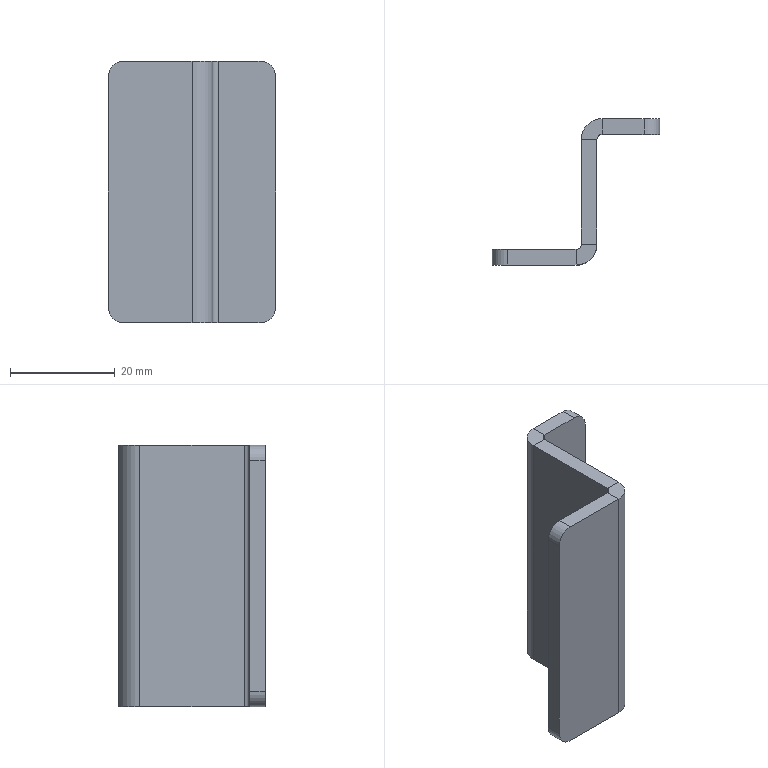Part | SolidWorks | features Fillet 1, FlatPattern 1, SMBaseFlange 1, SheetMetal 1 | 1 solid | 26 faces | box 32 x 28 x 50 mm | volume 8205 mm3 | plane 18 | cylinder 8 | commonest cylinder face diameters 6 x4 2 x2 8 x2
STEP:
#1=CARTESIAN_POINT('',(17.,1.,25.));
#2=VERTEX_POINT('',#1);
#3=CARTESIAN_POINT('',(20.,1.,25.));
#4=VERTEX_POINT('',#3);
#5=CARTESIAN_POINT('',(17.,1.,25.));
#6=DIRECTION('',(1.,0.,0.));
#7=VECTOR('',#6,1000.);
#8=LINE('',#5,#7);
#9=EDGE_CURVE('',#2,#4,#8,.T.);
#10=ORIENTED_EDGE('',*,*,#9,.F.);
#11=CARTESIAN_POINT('',(16.,0.,25.));
#12=VERTEX_POINT('',#11);
#13=CARTESIAN_POINT('',(16.,1.,25.));
#14=DIRECTION('',(0.,0.,1.));
#15=DIRECTION('',(-1.,0.,0.));
#16=AXIS2_PLACEMENT_3D('',#13,#14,#15);
#17=CIRCLE('',#16,1.);
#18=EDGE_CURVE('',#12,#2,#17,.T.);
#19=ORIENTED_EDGE('',*,*,#18,.F.);
#20=CARTESIAN_POINT('',(16.,-3.,25.));
#21=VERTEX_POINT('',#20);
#22=CARTESIAN_POINT('',(16.,-3.,25.));
#23=DIRECTION('',(0.,1.,0.));
#24=VECTOR('',#23,1000.);
#25=LINE('',#22,#24);
#26=EDGE_CURVE('',#21,#12,#25,.T.);
#27=ORIENTED_EDGE('',*,*,#26,.F.);
#28=CARTESIAN_POINT('',(16.,1.,25.));
#29=DIRECTION('',(0.,0.,1.));
#30=DIRECTION('',(1.,0.,0.));
#31=AXIS2_PLACEMENT_3D('',#28,#29,#30);
#32=CIRCLE('',#31,4.);
#33=EDGE_CURVE('',#21,#4,#32,.T.);
#34=ORIENTED_EDGE('',*,*,#33,.T.);
#35=EDGE_LOOP('',(#10,#19,#27,#34));
#36=FACE_OUTER_BOUND('',#35,.T.);
#37=CARTESIAN_POINT('',(17.,1.,25.));
#38=DIRECTION('',(0.,0.,1.));
#39=DIRECTION('',(1.,0.,0.));
#40=AXIS2_PLACEMENT_3D('',#37,#38,#39);
#41=PLANE('',#40);
#42=ADVANCED_FACE('',(#36),#41,.T.);
#43=CARTESIAN_POINT('',(17.,21.,25.));
#44=VERTEX_POINT('',#43);
#45=CARTESIAN_POINT('',(17.,0.,25.));
#46=DIRECTION('',(0.,1.,0.));
#47=VECTOR('',#46,1000.);
#48=LINE('',#45,#47);
#49=EDGE_CURVE('',#2,#44,#48,.T.);
#50=ORIENTED_EDGE('',*,*,#49,.F.);
#51=ORIENTED_EDGE('',*,*,#9,.T.);
#52=CARTESIAN_POINT('',(20.,21.,25.));
#53=VERTEX_POINT('',#52);
#54=CARTESIAN_POINT('',(20.,0.,25.));
#55=DIRECTION('',(0.,1.,0.));
#56=VECTOR('',#55,1000.);
#57=LINE('',#54,#56);
#58=EDGE_CURVE('',#4,#53,#57,.T.);
#59=ORIENTED_EDGE('',*,*,#58,.T.);
#60=CARTESIAN_POINT('',(20.,21.,25.));
#61=DIRECTION('',(-1.,0.,0.));
#62=VECTOR('',#61,1000.);
#63=LINE('',#60,#62);
#64=EDGE_CURVE('',#53,#44,#63,.T.);
#65=ORIENTED_EDGE('',*,*,#64,.T.);
#66=EDGE_LOOP('',(#50,#51,#59,#65));
#67=FACE_OUTER_BOUND('',#66,.T.);
#68=CARTESIAN_POINT('',(16.,-3.,25.));
#69=DIRECTION('',(0.,0.,1.));
#70=DIRECTION('',(1.,0.,0.));
#71=AXIS2_PLACEMENT_3D('',#68,#69,#70);
#72=PLANE('',#71);
#73=ADVANCED_FACE('',(#67),#72,.T.);
#74=CARTESIAN_POINT('',(16.,0.,-25.));
#75=VERTEX_POINT('',#74);
#76=CARTESIAN_POINT('',(16.,-3.,-25.));
#77=VERTEX_POINT('',#76);
#78=CARTESIAN_POINT('',(16.,0.,-25.));
#79=DIRECTION('',(0.,-1.,0.));
#80=VECTOR('',#79,1000.);
#81=LINE('',#78,#80);
#82=EDGE_CURVE('',#75,#77,#81,.T.);
#83=ORIENTED_EDGE('',*,*,#82,.F.);
#84=CARTESIAN_POINT('',(17.,1.,-25.));
#85=VERTEX_POINT('',#84);
#86=CARTESIAN_POINT('',(16.,1.,-25.));
#87=DIRECTION('',(0.,0.,1.));
#88=DIRECTION('',(-1.,0.,0.));
#89=AXIS2_PLACEMENT_3D('',#86,#87,#88);
#90=CIRCLE('',#89,1.);
#91=EDGE_CURVE('',#75,#85,#90,.T.);
#92=ORIENTED_EDGE('',*,*,#91,.T.);
#93=CARTESIAN_POINT('',(20.,1.,-25.));
#94=VERTEX_POINT('',#93);
#95=CARTESIAN_POINT('',(20.,1.,-25.));
#96=DIRECTION('',(-1.,0.,0.));
#97=VECTOR('',#96,1000.);
#98=LINE('',#95,#97);
#99=EDGE_CURVE('',#94,#85,#98,.T.);
#100=ORIENTED_EDGE('',*,*,#99,.F.);
#101=CARTESIAN_POINT('',(16.,1.,-25.));
#102=DIRECTION('',(0.,0.,1.));
#103=DIRECTION('',(1.,0.,0.));
#104=AXIS2_PLACEMENT_3D('',#101,#102,#103);
#105=CIRCLE('',#104,4.);
#106=EDGE_CURVE('',#77,#94,#105,.T.);
#107=ORIENTED_EDGE('',*,*,#106,.F.);
#108=EDGE_LOOP('',(#83,#92,#100,#107));
#109=FACE_OUTER_BOUND('',#108,.T.);
#110=CARTESIAN_POINT('',(16.,0.,-25.));
#111=DIRECTION('',(0.,0.,-1.));
#112=DIRECTION('',(-1.,0.,0.));
#113=AXIS2_PLACEMENT_3D('',#110,#111,#112);
#114=PLANE('',#113);
#115=ADVANCED_FACE('',(#109),#114,.T.);
#116=CARTESIAN_POINT('',(3.,-3.,-25.));
#117=VERTEX_POINT('',#116);
#118=CARTESIAN_POINT('',(0.,-3.,-25.));
#119=DIRECTION('',(1.,0.,0.));
#120=VECTOR('',#119,1000.);
#121=LINE('',#118,#120);
#122=EDGE_CURVE('',#117,#77,#121,.T.);
#123=ORIENTED_EDGE('',*,*,#122,.F.);
#124=CARTESIAN_POINT('',(3.,0.,-25.));
#125=VERTEX_POINT('',#124);
#126=CARTESIAN_POINT('',(3.,1.,-25.));
#127=DIRECTION('',(0.,1.,0.));
#128=VECTOR('',#127,1000.);
#129=LINE('',#126,#128);
#130=EDGE_CURVE('',#117,#125,#129,.T.);
#131=ORIENTED_EDGE('',*,*,#130,.T.);
#132=CARTESIAN_POINT('',(0.,0.,-25.));
#133=DIRECTION('',(1.,0.,0.));
#134=VECTOR('',#133,1000.);
#135=LINE('',#132,#134);
#136=EDGE_CURVE('',#125,#75,#135,.T.);
#137=ORIENTED_EDGE('',*,*,#136,.T.);
#138=ORIENTED_EDGE('',*,*,#82,.T.);
#139=EDGE_LOOP('',(#123,#131,#137,#138));
#140=FACE_OUTER_BOUND('',#139,.T.);
#141=CARTESIAN_POINT('',(20.,1.,-25.));
#142=DIRECTION('',(0.,0.,-1.));
#143=DIRECTION('',(-1.,0.,0.));
#144=AXIS2_PLACEMENT_3D('',#141,#142,#143);
#145=PLANE('',#144);
#146=ADVANCED_FACE('',(#140),#145,.T.);
#147=CARTESIAN_POINT('',(21.,25.,25.));
#148=VERTEX_POINT('',#147);
#149=CARTESIAN_POINT('',(21.,22.,25.));
#150=VERTEX_POINT('',#149);
#151=CARTESIAN_POINT('',(21.,25.,25.));
#152=DIRECTION('',(0.,-1.,0.));
#153=VECTOR('',#152,1000.);
#154=LINE('',#151,#153);
#155=EDGE_CURVE('',#148,#150,#154,.T.);
#156=ORIENTED_EDGE('',*,*,#155,.F.);
#157=CARTESIAN_POINT('',(21.,21.,25.));
#158=DIRECTION('',(0.,0.,-1.));
#159=DIRECTION('',(1.,0.,0.));
#160=AXIS2_PLACEMENT_3D('',#157,#158,#159);
#161=CIRCLE('',#160,4.);
#162=EDGE_CURVE('',#44,#148,#161,.T.);
#163=ORIENTED_EDGE('',*,*,#162,.F.);
#164=ORIENTED_EDGE('',*,*,#64,.F.);
#165=CARTESIAN_POINT('',(21.,21.,25.));
#166=DIRECTION('',(0.,0.,-1.));
#167=DIRECTION('',(1.,0.,0.));
#168=AXIS2_PLACEMENT_3D('',#165,#166,#167);
#169=CIRCLE('',#168,1.);
#170=EDGE_CURVE('',#53,#150,#169,.T.);
#171=ORIENTED_EDGE('',*,*,#170,.T.);
#172=EDGE_LOOP('',(#156,#163,#164,#171));
#173=FACE_OUTER_BOUND('',#172,.T.);
#174=CARTESIAN_POINT('',(21.,25.,25.));
#175=DIRECTION('',(0.,0.,1.));
#176=DIRECTION('',(1.,0.,0.));
#177=AXIS2_PLACEMENT_3D('',#174,#175,#176);
#178=PLANE('',#177);
#179=ADVANCED_FACE('',(#173),#178,.T.);
#180=CARTESIAN_POINT('',(29.,22.,25.));
#181=VERTEX_POINT('',#180);
#182=CARTESIAN_POINT('',(17.,22.,25.));
#183=DIRECTION('',(1.,0.,0.));
#184=VECTOR('',#183,1000.);
#185=LINE('',#182,#184);
#186=EDGE_CURVE('',#150,#181,#185,.T.);
#187=ORIENTED_EDGE('',*,*,#186,.T.);
#188=CARTESIAN_POINT('',(29.,25.,25.));
#189=VERTEX_POINT('',#188);
#190=CARTESIAN_POINT('',(29.,21.,25.));
#191=DIRECTION('',(0.,1.,0.));
#192=VECTOR('',#191,1000.);
#193=LINE('',#190,#192);
#194=EDGE_CURVE('',#181,#189,#193,.T.);
#195=ORIENTED_EDGE('',*,*,#194,.T.);
#196=CARTESIAN_POINT('',(17.,25.,25.));
#197=DIRECTION('',(1.,0.,0.));
#198=VECTOR('',#197,1000.);
#199=LINE('',#196,#198);
#200=EDGE_CURVE('',#148,#189,#199,.T.);
#201=ORIENTED_EDGE('',*,*,#200,.F.);
#202=ORIENTED_EDGE('',*,*,#155,.T.);
#203=EDGE_LOOP('',(#187,#195,#201,#202));
#204=FACE_OUTER_BOUND('',#203,.T.);
#205=CARTESIAN_POINT('',(20.,21.,25.));
#206=DIRECTION('',(0.,0.,1.));
#207=DIRECTION('',(1.,0.,0.));
#208=AXIS2_PLACEMENT_3D('',#205,#206,#207);
#209=PLANE('',#208);
#210=ADVANCED_FACE('',(#204),#209,.T.);
#211=CARTESIAN_POINT('',(17.,21.,-25.));
#212=VERTEX_POINT('',#211);
#213=CARTESIAN_POINT('',(20.,21.,-25.));
#214=VERTEX_POINT('',#213);
#215=CARTESIAN_POINT('',(17.,21.,-25.));
#216=DIRECTION('',(1.,0.,0.));
#217=VECTOR('',#216,1000.);
#218=LINE('',#215,#217);
#219=EDGE_CURVE('',#212,#214,#218,.T.);
#220=ORIENTED_EDGE('',*,*,#219,.F.);
#221=CARTESIAN_POINT('',(21.,25.,-25.));
#222=VERTEX_POINT('',#221);
#223=CARTESIAN_POINT('',(21.,21.,-25.));
#224=DIRECTION('',(0.,0.,-1.));
#225=DIRECTION('',(1.,0.,0.));
#226=AXIS2_PLACEMENT_3D('',#223,#224,#225);
#227=CIRCLE('',#226,4.);
#228=EDGE_CURVE('',#212,#222,#227,.T.);
#229=ORIENTED_EDGE('',*,*,#228,.T.);
#230=CARTESIAN_POINT('',(21.,22.,-25.));
#231=VERTEX_POINT('',#230);
#232=CARTESIAN_POINT('',(21.,22.,-25.));
#233=DIRECTION('',(0.,1.,0.));
#234=VECTOR('',#233,1000.);
#235=LINE('',#232,#234);
#236=EDGE_CURVE('',#231,#222,#235,.T.);
#237=ORIENTED_EDGE('',*,*,#236,.F.);
#238=CARTESIAN_POINT('',(21.,21.,-25.));
#239=DIRECTION('',(0.,0.,-1.));
#240=DIRECTION('',(1.,0.,0.));
#241=AXIS2_PLACEMENT_3D('',#238,#239,#240);
#242=CIRCLE('',#241,1.);
#243=EDGE_CURVE('',#214,#231,#242,.T.);
#244=ORIENTED_EDGE('',*,*,#243,.F.);
#245=EDGE_LOOP('',(#220,#229,#237,#244));
#246=FACE_OUTER_BOUND('',#245,.T.);
#247=CARTESIAN_POINT('',(17.,21.,-25.));
#248=DIRECTION('',(0.,0.,-1.));
#249=DIRECTION('',(-1.,0.,0.));
#250=AXIS2_PLACEMENT_3D('',#247,#248,#249);
#251=PLANE('',#250);
#252=ADVANCED_FACE('',(#246),#251,.T.);
#253=CARTESIAN_POINT('',(17.,0.,-25.));
#254=DIRECTION('',(0.,1.,0.));
#255=VECTOR('',#254,1000.);
#256=LINE('',#253,#255);
#257=EDGE_CURVE('',#85,#212,#256,.T.);
#258=ORIENTED_EDGE('',*,*,#257,.T.);
#259=ORIENTED_EDGE('',*,*,#219,.T.);
#260=CARTESIAN_POINT('',(20.,0.,-25.));
#261=DIRECTION('',(0.,1.,0.));
#262=VECTOR('',#261,1000.);
#263=LINE('',#260,#262);
#264=EDGE_CURVE('',#94,#214,#263,.T.);
#265=ORIENTED_EDGE('',*,*,#264,.F.);
#266=ORIENTED_EDGE('',*,*,#99,.T.);
#267=EDGE_LOOP('',(#258,#259,#265,#266));
#268=FACE_OUTER_BOUND('',#267,.T.);
#269=CARTESIAN_POINT('',(21.,22.,-25.));
#270=DIRECTION('',(0.,0.,-1.));
#271=DIRECTION('',(-1.,0.,0.));
#272=AXIS2_PLACEMENT_3D('',#269,#270,#271);
#273=PLANE('',#272);
#274=ADVANCED_FACE('',(#268),#273,.T.);
#275=CARTESIAN_POINT('',(29.,22.,-25.));
#276=VERTEX_POINT('',#275);
#277=CARTESIAN_POINT('',(17.,22.,-25.));
#278=DIRECTION('',(1.,0.,0.));
#279=VECTOR('',#278,1000.);
#280=LINE('',#277,#279);
#281=EDGE_CURVE('',#231,#276,#280,.T.);
#282=ORIENTED_EDGE('',*,*,#281,.T.);
#283=CARTESIAN_POINT('',(32.,22.,-22.));
#284=VERTEX_POINT('',#283);
#285=CARTESIAN_POINT('',(29.,22.,-22.));
#286=DIRECTION('',(0.,-1.,0.));
#287=DIRECTION('',(0.,0.,1.));
#288=AXIS2_PLACEMENT_3D('',#285,#286,#287);
#289=CIRCLE('',#288,3.);
#290=EDGE_CURVE('',#276,#284,#289,.T.);
#291=ORIENTED_EDGE('',*,*,#290,.T.);
#292=CARTESIAN_POINT('',(32.,22.,22.));
#293=VERTEX_POINT('',#292);
#294=CARTESIAN_POINT('',(32.,22.,25.));
#295=DIRECTION('',(0.,0.,-1.));
#296=VECTOR('',#295,1000.);
#297=LINE('',#294,#296);
#298=EDGE_CURVE('',#293,#284,#297,.T.);
#299=ORIENTED_EDGE('',*,*,#298,.F.);
#300=CARTESIAN_POINT('',(29.,22.,22.));
#301=DIRECTION('',(0.,-1.,0.));
#302=DIRECTION('',(0.,0.,1.));
#303=AXIS2_PLACEMENT_3D('',#300,#301,#302);
#304=CIRCLE('',#303,3.);
#305=EDGE_CURVE('',#293,#181,#304,.T.);
#306=ORIENTED_EDGE('',*,*,#305,.T.);
#307=ORIENTED_EDGE('',*,*,#186,.F.);
#308=CARTESIAN_POINT('',(21.,22.,25.));
#309=DIRECTION('',(0.,0.,-1.));
#310=VECTOR('',#309,1000.);
#311=LINE('',#308,#310);
#312=EDGE_CURVE('',#150,#231,#311,.T.);
#313=ORIENTED_EDGE('',*,*,#312,.T.);
#314=EDGE_LOOP('',(#282,#291,#299,#306,#307,#313));
#315=FACE_OUTER_BOUND('',#314,.T.);
#316=CARTESIAN_POINT('',(17.,22.,25.));
#317=DIRECTION('',(0.,1.,0.));
#318=DIRECTION('',(0.,0.,1.));
#319=AXIS2_PLACEMENT_3D('',#316,#317,#318);
#320=PLANE('',#319);
#321=ADVANCED_FACE('',(#315),#320,.F.);
#322=ORIENTED_EDGE('',*,*,#298,.T.);
#323=CARTESIAN_POINT('',(32.,25.,-22.));
#324=VERTEX_POINT('',#323);
#325=CARTESIAN_POINT('',(32.,25.,-22.));
#326=DIRECTION('',(0.,1.,0.));
#327=VECTOR('',#326,1000.);
#328=LINE('',#325,#327);
#329=EDGE_CURVE('',#284,#324,#328,.T.);
#330=ORIENTED_EDGE('',*,*,#329,.T.);
#331=CARTESIAN_POINT('',(32.,25.,22.));
#332=VERTEX_POINT('',#331);
#333=CARTESIAN_POINT('',(32.,25.,25.));
#334=DIRECTION('',(0.,0.,-1.));
#335=VECTOR('',#334,1000.);
#336=LINE('',#333,#335);
#337=EDGE_CURVE('',#332,#324,#336,.T.);
#338=ORIENTED_EDGE('',*,*,#337,.F.);
#339=CARTESIAN_POINT('',(32.,25.,22.));
#340=DIRECTION('',(0.,-1.,0.));
#341=VECTOR('',#340,1000.);
#342=LINE('',#339,#341);
#343=EDGE_CURVE('',#332,#293,#342,.T.);
#344=ORIENTED_EDGE('',*,*,#343,.T.);
#345=EDGE_LOOP('',(#322,#330,#338,#344));
#346=FACE_OUTER_BOUND('',#345,.T.);
#347=CARTESIAN_POINT('',(32.,25.,25.));
#348=DIRECTION('',(1.,0.,0.));
#349=DIRECTION('',(0.,0.,-1.));
#350=AXIS2_PLACEMENT_3D('',#347,#348,#349);
#351=PLANE('',#350);
#352=ADVANCED_FACE('',(#346),#351,.T.);
#353=ORIENTED_EDGE('',*,*,#337,.T.);
#354=CARTESIAN_POINT('',(29.,25.,-25.));
#355=VERTEX_POINT('',#354);
#356=CARTESIAN_POINT('',(29.,25.,-22.));
#357=DIRECTION('',(0.,1.,0.));
#358=DIRECTION('',(0.,0.,1.));
#359=AXIS2_PLACEMENT_3D('',#356,#357,#358);
#360=CIRCLE('',#359,3.);
#361=EDGE_CURVE('',#324,#355,#360,.T.);
#362=ORIENTED_EDGE('',*,*,#361,.T.);
#363=CARTESIAN_POINT('',(17.,25.,-25.));
#364=DIRECTION('',(1.,0.,0.));
#365=VECTOR('',#364,1000.);
#366=LINE('',#363,#365);
#367=EDGE_CURVE('',#222,#355,#366,.T.);
#368=ORIENTED_EDGE('',*,*,#367,.F.);
#369=CARTESIAN_POINT('',(21.,25.,25.));
#370=DIRECTION('',(0.,0.,-1.));
#371=VECTOR('',#370,1000.);
#372=LINE('',#369,#371);
#373=EDGE_CURVE('',#148,#222,#372,.T.);
#374=ORIENTED_EDGE('',*,*,#373,.F.);
#375=ORIENTED_EDGE('',*,*,#200,.T.);
#376=CARTESIAN_POINT('',(29.,25.,22.));
#377=DIRECTION('',(0.,1.,0.));
#378=DIRECTION('',(0.,0.,1.));
#379=AXIS2_PLACEMENT_3D('',#376,#377,#378);
#380=CIRCLE('',#379,3.);
#381=EDGE_CURVE('',#189,#332,#380,.T.);
#382=ORIENTED_EDGE('',*,*,#381,.T.);
#383=EDGE_LOOP('',(#353,#362,#368,#374,#375,#382));
#384=FACE_OUTER_BOUND('',#383,.T.);
#385=CARTESIAN_POINT('',(17.,25.,25.));
#386=DIRECTION('',(0.,1.,0.));
#387=DIRECTION('',(0.,0.,1.));
#388=AXIS2_PLACEMENT_3D('',#385,#386,#387);
#389=PLANE('',#388);
#390=ADVANCED_FACE('',(#384),#389,.T.);
#391=ORIENTED_EDGE('',*,*,#228,.F.);
#392=CARTESIAN_POINT('',(17.,21.,25.));
#393=DIRECTION('',(0.,0.,-1.));
#394=VECTOR('',#393,1000.);
#395=LINE('',#392,#394);
#396=EDGE_CURVE('',#44,#212,#395,.T.);
#397=ORIENTED_EDGE('',*,*,#396,.F.);
#398=ORIENTED_EDGE('',*,*,#162,.T.);
#399=ORIENTED_EDGE('',*,*,#373,.T.);
#400=EDGE_LOOP('',(#391,#397,#398,#399));
#401=FACE_OUTER_BOUND('',#400,.T.);
#402=CARTESIAN_POINT('',(21.,21.,25.));
#403=DIRECTION('',(0.,0.,-1.));
#404=DIRECTION('',(-1.,0.,0.));
#405=AXIS2_PLACEMENT_3D('',#402,#403,#404);
#406=CYLINDRICAL_SURFACE('',#405,4.);
#407=ADVANCED_FACE('',(#401),#406,.T.);
#408=ORIENTED_EDGE('',*,*,#257,.F.);
#409=CARTESIAN_POINT('',(17.,1.,25.));
#410=DIRECTION('',(0.,0.,-1.));
#411=VECTOR('',#410,1000.);
#412=LINE('',#409,#411);
#413=EDGE_CURVE('',#2,#85,#412,.T.);
#414=ORIENTED_EDGE('',*,*,#413,.F.);
#415=ORIENTED_EDGE('',*,*,#49,.T.);
#416=ORIENTED_EDGE('',*,*,#396,.T.);
#417=EDGE_LOOP('',(#408,#414,#415,#416));
#418=FACE_OUTER_BOUND('',#417,.T.);
#419=CARTESIAN_POINT('',(17.,0.,25.));
#420=DIRECTION('',(-1.,0.,0.));
#421=DIRECTION('',(0.,0.,1.));
#422=AXIS2_PLACEMENT_3D('',#419,#420,#421);
#423=PLANE('',#422);
#424=ADVANCED_FACE('',(#418),#423,.T.);
#425=ORIENTED_EDGE('',*,*,#91,.F.);
#426=CARTESIAN_POINT('',(16.,0.,25.));
#427=DIRECTION('',(0.,0.,-1.));
#428=VECTOR('',#427,1000.);
#429=LINE('',#426,#428);
#430=EDGE_CURVE('',#12,#75,#429,.T.);
#431=ORIENTED_EDGE('',*,*,#430,.F.);
#432=ORIENTED_EDGE('',*,*,#18,.T.);
#433=ORIENTED_EDGE('',*,*,#413,.T.);
#434=EDGE_LOOP('',(#425,#431,#432,#433));
#435=FACE_OUTER_BOUND('',#434,.T.);
#436=CARTESIAN_POINT('',(16.,1.,25.));
#437=DIRECTION('',(0.,0.,-1.));
#438=DIRECTION('',(-1.,0.,0.));
#439=AXIS2_PLACEMENT_3D('',#436,#437,#438);
#440=CYLINDRICAL_SURFACE('',#439,1.);
#441=ADVANCED_FACE('',(#435),#440,.F.);
#442=CARTESIAN_POINT('',(0.,0.,22.));
#443=VERTEX_POINT('',#442);
#444=CARTESIAN_POINT('',(0.,0.,-22.));
#445=VERTEX_POINT('',#444);
#446=CARTESIAN_POINT('',(0.,0.,25.));
#447=DIRECTION('',(0.,0.,-1.));
#448=VECTOR('',#447,1000.);
#449=LINE('',#446,#448);
#450=EDGE_CURVE('',#443,#445,#449,.T.);
#451=ORIENTED_EDGE('',*,*,#450,.F.);
#452=CARTESIAN_POINT('',(3.,0.,25.));
#453=VERTEX_POINT('',#452);
#454=CARTESIAN_POINT('',(3.,0.,22.));
#455=DIRECTION('',(0.,1.,0.));
#456=DIRECTION('',(0.,0.,1.));
#457=AXIS2_PLACEMENT_3D('',#454,#455,#456);
#458=CIRCLE('',#457,3.);
#459=EDGE_CURVE('',#443,#453,#458,.T.);
#460=ORIENTED_EDGE('',*,*,#459,.T.);
#461=CARTESIAN_POINT('',(0.,0.,25.));
#462=DIRECTION('',(1.,0.,0.));
#463=VECTOR('',#462,1000.);
#464=LINE('',#461,#463);
#465=EDGE_CURVE('',#453,#12,#464,.T.);
#466=ORIENTED_EDGE('',*,*,#465,.T.);
#467=ORIENTED_EDGE('',*,*,#430,.T.);
#468=ORIENTED_EDGE('',*,*,#136,.F.);
#469=CARTESIAN_POINT('',(3.,0.,-22.));
#470=DIRECTION('',(0.,1.,0.));
#471=DIRECTION('',(0.,0.,1.));
#472=AXIS2_PLACEMENT_3D('',#469,#470,#471);
#473=CIRCLE('',#472,3.);
#474=EDGE_CURVE('',#125,#445,#473,.T.);
#475=ORIENTED_EDGE('',*,*,#474,.T.);
#476=EDGE_LOOP('',(#451,#460,#466,#467,#468,#475));
#477=FACE_OUTER_BOUND('',#476,.T.);
#478=CARTESIAN_POINT('',(0.,0.,25.));
#479=DIRECTION('',(0.,1.,0.));
#480=DIRECTION('',(0.,0.,1.));
#481=AXIS2_PLACEMENT_3D('',#478,#479,#480);
#482=PLANE('',#481);
#483=ADVANCED_FACE('',(#477),#482,.T.);
#484=CARTESIAN_POINT('',(0.,-3.,22.));
#485=VERTEX_POINT('',#484);
#486=CARTESIAN_POINT('',(0.,-3.,-22.));
#487=VERTEX_POINT('',#486);
#488=CARTESIAN_POINT('',(0.,-3.,25.));
#489=DIRECTION('',(0.,0.,-1.));
#490=VECTOR('',#489,1000.);
#491=LINE('',#488,#490);
#492=EDGE_CURVE('',#485,#487,#491,.T.);
#493=ORIENTED_EDGE('',*,*,#492,.F.);
#494=CARTESIAN_POINT('',(0.,-3.,22.));
#495=DIRECTION('',(0.,1.,0.));
#496=VECTOR('',#495,1000.);
#497=LINE('',#494,#496);
#498=EDGE_CURVE('',#485,#443,#497,.T.);
#499=ORIENTED_EDGE('',*,*,#498,.T.);
#500=ORIENTED_EDGE('',*,*,#450,.T.);
#501=CARTESIAN_POINT('',(0.,-3.,-22.));
#502=DIRECTION('',(0.,-1.,0.));
#503=VECTOR('',#502,1000.);
#504=LINE('',#501,#503);
#505=EDGE_CURVE('',#445,#487,#504,.T.);
#506=ORIENTED_EDGE('',*,*,#505,.T.);
#507=EDGE_LOOP('',(#493,#499,#500,#506));
#508=FACE_OUTER_BOUND('',#507,.T.);
#509=CARTESIAN_POINT('',(0.,-3.,25.));
#510=DIRECTION('',(-1.,0.,0.));
#511=DIRECTION('',(0.,0.,1.));
#512=AXIS2_PLACEMENT_3D('',#509,#510,#511);
#513=PLANE('',#512);
#514=ADVANCED_FACE('',(#508),#513,.T.);
#515=CARTESIAN_POINT('',(3.,-3.,25.));
#516=VERTEX_POINT('',#515);
#517=CARTESIAN_POINT('',(0.,-3.,25.));
#518=DIRECTION('',(1.,0.,0.));
#519=VECTOR('',#518,1000.);
#520=LINE('',#517,#519);
#521=EDGE_CURVE('',#516,#21,#520,.T.);
#522=ORIENTED_EDGE('',*,*,#521,.F.);
#523=CARTESIAN_POINT('',(3.,-3.,22.));
#524=DIRECTION('',(0.,-1.,0.));
#525=DIRECTION('',(0.,0.,1.));
#526=AXIS2_PLACEMENT_3D('',#523,#524,#525);
#527=CIRCLE('',#526,3.);
#528=EDGE_CURVE('',#516,#485,#527,.T.);
#529=ORIENTED_EDGE('',*,*,#528,.T.);
#530=ORIENTED_EDGE('',*,*,#492,.T.);
#531=CARTESIAN_POINT('',(3.,-3.,-22.));
#532=DIRECTION('',(0.,-1.,0.));
#533=DIRECTION('',(0.,0.,1.));
#534=AXIS2_PLACEMENT_3D('',#531,#532,#533);
#535=CIRCLE('',#534,3.);
#536=EDGE_CURVE('',#487,#117,#535,.T.);
#537=ORIENTED_EDGE('',*,*,#536,.T.);
#538=ORIENTED_EDGE('',*,*,#122,.T.);
#539=CARTESIAN_POINT('',(16.,-3.,25.));
#540=DIRECTION('',(0.,0.,-1.));
#541=VECTOR('',#540,1000.);
#542=LINE('',#539,#541);
#543=EDGE_CURVE('',#21,#77,#542,.T.);
#544=ORIENTED_EDGE('',*,*,#543,.F.);
#545=EDGE_LOOP('',(#522,#529,#530,#537,#538,#544));
#546=FACE_OUTER_BOUND('',#545,.T.);
#547=CARTESIAN_POINT('',(0.,-3.,25.));
#548=DIRECTION('',(0.,1.,0.));
#549=DIRECTION('',(0.,0.,1.));
#550=AXIS2_PLACEMENT_3D('',#547,#548,#549);
#551=PLANE('',#550);
#552=ADVANCED_FACE('',(#546),#551,.F.);
#553=ORIENTED_EDGE('',*,*,#106,.T.);
#554=CARTESIAN_POINT('',(20.,1.,25.));
#555=DIRECTION('',(0.,0.,-1.));
#556=VECTOR('',#555,1000.);
#557=LINE('',#554,#556);
#558=EDGE_CURVE('',#4,#94,#557,.T.);
#559=ORIENTED_EDGE('',*,*,#558,.F.);
#560=ORIENTED_EDGE('',*,*,#33,.F.);
#561=ORIENTED_EDGE('',*,*,#543,.T.);
#562=EDGE_LOOP('',(#553,#559,#560,#561));
#563=FACE_OUTER_BOUND('',#562,.T.);
#564=CARTESIAN_POINT('',(16.,1.,25.));
#565=DIRECTION('',(0.,0.,-1.));
#566=DIRECTION('',(-1.,0.,0.));
#567=AXIS2_PLACEMENT_3D('',#564,#565,#566);
#568=CYLINDRICAL_SURFACE('',#567,4.);
#569=ADVANCED_FACE('',(#563),#568,.T.);
#570=ORIENTED_EDGE('',*,*,#264,.T.);
#571=CARTESIAN_POINT('',(20.,21.,25.));
#572=DIRECTION('',(0.,0.,-1.));
#573=VECTOR('',#572,1000.);
#574=LINE('',#571,#573);
#575=EDGE_CURVE('',#53,#214,#574,.T.);
#576=ORIENTED_EDGE('',*,*,#575,.F.);
#577=ORIENTED_EDGE('',*,*,#58,.F.);
#578=ORIENTED_EDGE('',*,*,#558,.T.);
#579=EDGE_LOOP('',(#570,#576,#577,#578));
#580=FACE_OUTER_BOUND('',#579,.T.);
#581=CARTESIAN_POINT('',(20.,0.,25.));
#582=DIRECTION('',(-1.,0.,0.));
#583=DIRECTION('',(0.,0.,1.));
#584=AXIS2_PLACEMENT_3D('',#581,#582,#583);
#585=PLANE('',#584);
#586=ADVANCED_FACE('',(#580),#585,.F.);
#587=ORIENTED_EDGE('',*,*,#243,.T.);
#588=ORIENTED_EDGE('',*,*,#312,.F.);
#589=ORIENTED_EDGE('',*,*,#170,.F.);
#590=ORIENTED_EDGE('',*,*,#575,.T.);
#591=EDGE_LOOP('',(#587,#588,#589,#590));
#592=FACE_OUTER_BOUND('',#591,.T.);
#593=CARTESIAN_POINT('',(21.,21.,25.));
#594=DIRECTION('',(0.,0.,-1.));
#595=DIRECTION('',(-1.,0.,0.));
#596=AXIS2_PLACEMENT_3D('',#593,#594,#595);
#597=CYLINDRICAL_SURFACE('',#596,1.);
#598=ADVANCED_FACE('',(#592),#597,.F.);
#599=ORIENTED_EDGE('',*,*,#465,.F.);
#600=CARTESIAN_POINT('',(3.,21.,25.));
#601=DIRECTION('',(0.,-1.,0.));
#602=VECTOR('',#601,1000.);
#603=LINE('',#600,#602);
#604=EDGE_CURVE('',#453,#516,#603,.T.);
#605=ORIENTED_EDGE('',*,*,#604,.T.);
#606=ORIENTED_EDGE('',*,*,#521,.T.);
#607=ORIENTED_EDGE('',*,*,#26,.T.);
#608=EDGE_LOOP('',(#599,#605,#606,#607));
#609=FACE_OUTER_BOUND('',#608,.T.);
#610=CARTESIAN_POINT('',(21.,21.,25.));
#611=DIRECTION('',(0.,0.,1.));
#612=DIRECTION('',(1.,0.,0.));
#613=AXIS2_PLACEMENT_3D('',#610,#611,#612);
#614=PLANE('',#613);
#615=ADVANCED_FACE('',(#609),#614,.T.);
#616=ORIENTED_EDGE('',*,*,#367,.T.);
#617=CARTESIAN_POINT('',(29.,22.,-25.));
#618=DIRECTION('',(0.,-1.,0.));
#619=VECTOR('',#618,1000.);
#620=LINE('',#617,#619);
#621=EDGE_CURVE('',#355,#276,#620,.T.);
#622=ORIENTED_EDGE('',*,*,#621,.T.);
#623=ORIENTED_EDGE('',*,*,#281,.F.);
#624=ORIENTED_EDGE('',*,*,#236,.T.);
#625=EDGE_LOOP('',(#616,#622,#623,#624));
#626=FACE_OUTER_BOUND('',#625,.T.);
#627=CARTESIAN_POINT('',(21.,21.,-25.));
#628=DIRECTION('',(0.,0.,1.));
#629=DIRECTION('',(1.,0.,0.));
#630=AXIS2_PLACEMENT_3D('',#627,#628,#629);
#631=PLANE('',#630);
#632=ADVANCED_FACE('',(#626),#631,.F.);
#633=ORIENTED_EDGE('',*,*,#528,.F.);
#634=ORIENTED_EDGE('',*,*,#604,.F.);
#635=ORIENTED_EDGE('',*,*,#459,.F.);
#636=ORIENTED_EDGE('',*,*,#498,.F.);
#637=EDGE_LOOP('',(#633,#634,#635,#636));
#638=FACE_OUTER_BOUND('',#637,.T.);
#639=CARTESIAN_POINT('',(3.,-3.,22.));
#640=DIRECTION('',(0.,1.,0.));
#641=DIRECTION('',(0.,0.,1.));
#642=AXIS2_PLACEMENT_3D('',#639,#640,#641);
#643=CYLINDRICAL_SURFACE('',#642,3.);
#644=ADVANCED_FACE('',(#638),#643,.T.);
#645=ORIENTED_EDGE('',*,*,#536,.F.);
#646=ORIENTED_EDGE('',*,*,#505,.F.);
#647=ORIENTED_EDGE('',*,*,#474,.F.);
#648=ORIENTED_EDGE('',*,*,#130,.F.);
#649=EDGE_LOOP('',(#645,#646,#647,#648));
#650=FACE_OUTER_BOUND('',#649,.T.);
#651=CARTESIAN_POINT('',(3.,1.,-22.));
#652=DIRECTION('',(0.,1.,0.));
#653=DIRECTION('',(0.,0.,1.));
#654=AXIS2_PLACEMENT_3D('',#651,#652,#653);
#655=CYLINDRICAL_SURFACE('',#654,3.);
#656=ADVANCED_FACE('',(#650),#655,.T.);
#657=ORIENTED_EDGE('',*,*,#361,.F.);
#658=ORIENTED_EDGE('',*,*,#329,.F.);
#659=ORIENTED_EDGE('',*,*,#290,.F.);
#660=ORIENTED_EDGE('',*,*,#621,.F.);
#661=EDGE_LOOP('',(#657,#658,#659,#660));
#662=FACE_OUTER_BOUND('',#661,.T.);
#663=CARTESIAN_POINT('',(29.,21.,-22.));
#664=DIRECTION('',(0.,1.,0.));
#665=DIRECTION('',(0.,0.,1.));
#666=AXIS2_PLACEMENT_3D('',#663,#664,#665);
#667=CYLINDRICAL_SURFACE('',#666,3.);
#668=ADVANCED_FACE('',(#662),#667,.T.);
#669=ORIENTED_EDGE('',*,*,#381,.F.);
#670=ORIENTED_EDGE('',*,*,#194,.F.);
#671=ORIENTED_EDGE('',*,*,#305,.F.);
#672=ORIENTED_EDGE('',*,*,#343,.F.);
#673=EDGE_LOOP('',(#669,#670,#671,#672));
#674=FACE_OUTER_BOUND('',#673,.T.);
#675=CARTESIAN_POINT('',(29.,25.,22.));
#676=DIRECTION('',(0.,-1.,0.));
#677=DIRECTION('',(0.,0.,-1.));
#678=AXIS2_PLACEMENT_3D('',#675,#676,#677);
#679=CYLINDRICAL_SURFACE('',#678,3.);
#680=ADVANCED_FACE('',(#674),#679,.T.);
#681=CLOSED_SHELL('',(#42,#73,#115,#146,#179,#210,#252,#274,#321,#352,#390,#407,#424,#441,#483,#514,#552,#569,#586,#598,#615,#632,#644,#656,#668,#680));
#682=MANIFOLD_SOLID_BREP('',#681);
#683=CARTESIAN_POINT('',(0.,0.,0.));
#684=DIRECTION('',(0.,0.,1.));
#685=DIRECTION('',(1.,0.,0.));
#686=AXIS2_PLACEMENT_3D('',#683,#684,#685);
#687=(LENGTH_UNIT()NAMED_UNIT(*)SI_UNIT(.MILLI.,.METRE.));
#688=UNCERTAINTY_MEASURE_WITH_UNIT(LENGTH_MEASURE(0.00001),#687,'','');
#689=(NAMED_UNIT(*)PLANE_ANGLE_UNIT()SI_UNIT($,.RADIAN.));
#690=(NAMED_UNIT(*)SI_UNIT($,.STERADIAN.)SOLID_ANGLE_UNIT());
#691=(GEOMETRIC_REPRESENTATION_CONTEXT(3)GLOBAL_UNCERTAINTY_ASSIGNED_CONTEXT((#688))GLOBAL_UNIT_ASSIGNED_CONTEXT((#687,#689,#690))REPRESENTATION_CONTEXT('',''));
#692=ADVANCED_BREP_SHAPE_REPRESENTATION('',(#682,#686),#691);